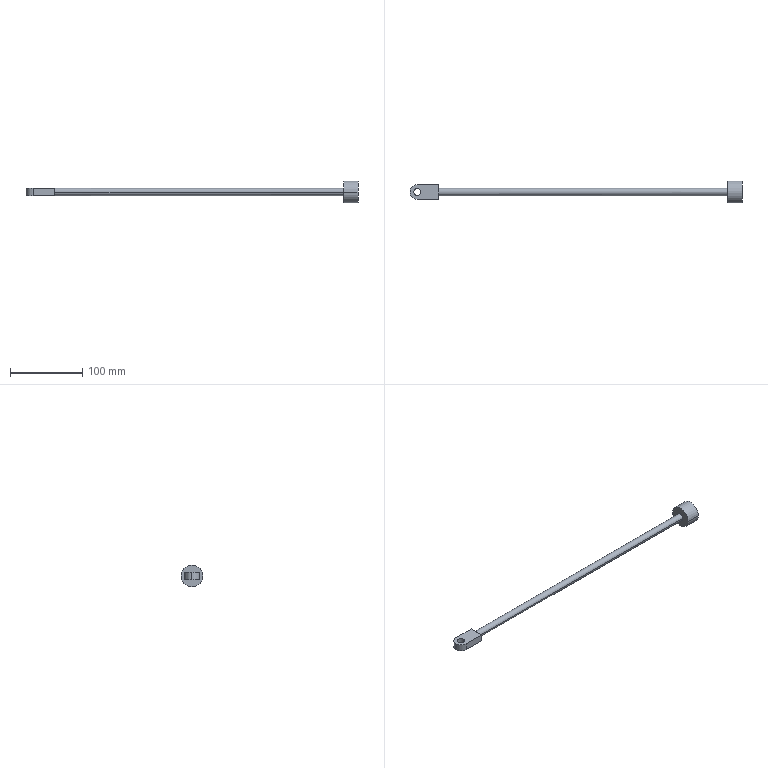Part | SolidWorks | features Extrusion 1, Revolution 1 | 1 solid | 16 faces | box 460 x 30 x 30 mm | volume 52338 mm3 | cylinder 8 | plane 8 | commonest cylinder face diameters 10 x4 20 x2 30 x2
STEP:
#1=CARTESIAN_POINT('',(430.,15.,0.));
#2=VERTEX_POINT('',#1);
#3=CARTESIAN_POINT('',(430.,-15.,0.));
#4=VERTEX_POINT('',#3);
#5=CARTESIAN_POINT('',(430.,0.,0.));
#6=DIRECTION('',(1.,0.,0.));
#7=DIRECTION('',(0.,1.,0.));
#8=AXIS2_PLACEMENT_3D('',#5,#6,#7);
#9=CIRCLE('',#8,15.);
#10=EDGE_CURVE('',#2,#4,#9,.T.);
#11=ORIENTED_EDGE('',*,*,#10,.T.);
#12=CARTESIAN_POINT('',(450.,-15.,0.));
#13=VERTEX_POINT('',#12);
#14=CARTESIAN_POINT('',(450.,-15.,0.));
#15=DIRECTION('',(1.,0.,0.));
#16=VECTOR('',#15,1000.);
#17=LINE('',#14,#16);
#18=EDGE_CURVE('',#4,#13,#17,.T.);
#19=ORIENTED_EDGE('',*,*,#18,.T.);
#20=CARTESIAN_POINT('',(450.,15.,0.));
#21=VERTEX_POINT('',#20);
#22=CARTESIAN_POINT('',(450.,0.,0.));
#23=DIRECTION('',(1.,0.,0.));
#24=DIRECTION('',(0.,1.,0.));
#25=AXIS2_PLACEMENT_3D('',#22,#23,#24);
#26=CIRCLE('',#25,15.);
#27=EDGE_CURVE('',#21,#13,#26,.T.);
#28=ORIENTED_EDGE('',*,*,#27,.F.);
#29=CARTESIAN_POINT('',(450.,15.,0.));
#30=DIRECTION('',(1.,0.,0.));
#31=VECTOR('',#30,1000.);
#32=LINE('',#29,#31);
#33=EDGE_CURVE('',#2,#21,#32,.T.);
#34=ORIENTED_EDGE('',*,*,#33,.F.);
#35=EDGE_LOOP('',(#11,#19,#28,#34));
#36=FACE_OUTER_BOUND('',#35,.T.);
#37=CARTESIAN_POINT('',(450.,0.,0.));
#38=DIRECTION('',(1.,0.,0.));
#39=DIRECTION('',(0.,1.,0.));
#40=AXIS2_PLACEMENT_3D('',#37,#38,#39);
#41=CYLINDRICAL_SURFACE('',#40,15.);
#42=ADVANCED_FACE('',(#36),#41,.T.);
#43=CARTESIAN_POINT('',(30.,0.,5.));
#44=VERTEX_POINT('',#43);
#45=CARTESIAN_POINT('',(30.,-5.,0.));
#46=VERTEX_POINT('',#45);
#47=CARTESIAN_POINT('',(30.,0.,0.));
#48=DIRECTION('',(1.,0.,0.));
#49=DIRECTION('',(0.,1.,0.));
#50=AXIS2_PLACEMENT_3D('',#47,#48,#49);
#51=CIRCLE('',#50,5.);
#52=EDGE_CURVE('',#44,#46,#51,.T.);
#53=ORIENTED_EDGE('',*,*,#52,.T.);
#54=CARTESIAN_POINT('',(430.,-5.,0.));
#55=VERTEX_POINT('',#54);
#56=CARTESIAN_POINT('',(450.,-5.,0.));
#57=DIRECTION('',(1.,0.,0.));
#58=VECTOR('',#57,1000.);
#59=LINE('',#56,#58);
#60=EDGE_CURVE('',#46,#55,#59,.T.);
#61=ORIENTED_EDGE('',*,*,#60,.T.);
#62=CARTESIAN_POINT('',(430.,5.,0.));
#63=VERTEX_POINT('',#62);
#64=CARTESIAN_POINT('',(430.,0.,0.));
#65=DIRECTION('',(1.,0.,0.));
#66=DIRECTION('',(0.,1.,0.));
#67=AXIS2_PLACEMENT_3D('',#64,#65,#66);
#68=CIRCLE('',#67,5.);
#69=EDGE_CURVE('',#63,#55,#68,.T.);
#70=ORIENTED_EDGE('',*,*,#69,.F.);
#71=CARTESIAN_POINT('',(30.,5.,0.));
#72=VERTEX_POINT('',#71);
#73=CARTESIAN_POINT('',(450.,5.,0.));
#74=DIRECTION('',(1.,0.,0.));
#75=VECTOR('',#74,1000.);
#76=LINE('',#73,#75);
#77=EDGE_CURVE('',#72,#63,#76,.T.);
#78=ORIENTED_EDGE('',*,*,#77,.F.);
#79=CARTESIAN_POINT('',(30.,0.,0.));
#80=DIRECTION('',(1.,0.,0.));
#81=DIRECTION('',(0.,1.,0.));
#82=AXIS2_PLACEMENT_3D('',#79,#80,#81);
#83=CIRCLE('',#82,5.);
#84=EDGE_CURVE('',#72,#44,#83,.T.);
#85=ORIENTED_EDGE('',*,*,#84,.T.);
#86=EDGE_LOOP('',(#53,#61,#70,#78,#85));
#87=FACE_OUTER_BOUND('',#86,.T.);
#88=CARTESIAN_POINT('',(450.,0.,0.));
#89=DIRECTION('',(1.,0.,0.));
#90=DIRECTION('',(0.,1.,0.));
#91=AXIS2_PLACEMENT_3D('',#88,#89,#90);
#92=CYLINDRICAL_SURFACE('',#91,5.);
#93=ADVANCED_FACE('',(#87),#92,.T.);
#94=CARTESIAN_POINT('',(-5.,0.,5.));
#95=VERTEX_POINT('',#94);
#96=CARTESIAN_POINT('',(5.,0.,5.));
#97=VERTEX_POINT('',#96);
#98=CARTESIAN_POINT('',(0.,0.,5.));
#99=DIRECTION('',(0.,0.,1.));
#100=DIRECTION('',(1.,0.,0.));
#101=AXIS2_PLACEMENT_3D('',#98,#99,#100);
#102=CIRCLE('',#101,5.);
#103=EDGE_CURVE('',#95,#97,#102,.T.);
#104=ORIENTED_EDGE('',*,*,#103,.T.);
#105=CARTESIAN_POINT('',(5.,0.,-5.));
#106=VERTEX_POINT('',#105);
#107=CARTESIAN_POINT('',(5.,0.,5.));
#108=DIRECTION('',(0.,0.,-1.));
#109=VECTOR('',#108,1000.);
#110=LINE('',#107,#109);
#111=EDGE_CURVE('',#97,#106,#110,.T.);
#112=ORIENTED_EDGE('',*,*,#111,.T.);
#113=CARTESIAN_POINT('',(-5.,0.,-5.));
#114=VERTEX_POINT('',#113);
#115=CARTESIAN_POINT('',(0.,0.,-5.));
#116=DIRECTION('',(0.,0.,1.));
#117=DIRECTION('',(1.,0.,0.));
#118=AXIS2_PLACEMENT_3D('',#115,#116,#117);
#119=CIRCLE('',#118,5.);
#120=EDGE_CURVE('',#114,#106,#119,.T.);
#121=ORIENTED_EDGE('',*,*,#120,.F.);
#122=CARTESIAN_POINT('',(-5.,0.,5.));
#123=DIRECTION('',(0.,0.,-1.));
#124=VECTOR('',#123,1000.);
#125=LINE('',#122,#124);
#126=EDGE_CURVE('',#95,#114,#125,.T.);
#127=ORIENTED_EDGE('',*,*,#126,.F.);
#128=EDGE_LOOP('',(#104,#112,#121,#127));
#129=FACE_OUTER_BOUND('',#128,.T.);
#130=CARTESIAN_POINT('',(0.,0.,5.));
#131=DIRECTION('',(0.,0.,-1.));
#132=DIRECTION('',(-1.,0.,0.));
#133=AXIS2_PLACEMENT_3D('',#130,#131,#132);
#134=CYLINDRICAL_SURFACE('',#133,5.);
#135=ADVANCED_FACE('',(#129),#134,.F.);
#136=CARTESIAN_POINT('',(-10.,0.,5.));
#137=VERTEX_POINT('',#136);
#138=CARTESIAN_POINT('',(0.,-10.,5.));
#139=VERTEX_POINT('',#138);
#140=CARTESIAN_POINT('',(0.,0.,5.));
#141=DIRECTION('',(0.,0.,1.));
#142=DIRECTION('',(1.,0.,0.));
#143=AXIS2_PLACEMENT_3D('',#140,#141,#142);
#144=CIRCLE('',#143,10.);
#145=EDGE_CURVE('',#137,#139,#144,.T.);
#146=ORIENTED_EDGE('',*,*,#145,.F.);
#147=CARTESIAN_POINT('',(-10.,0.,-5.));
#148=VERTEX_POINT('',#147);
#149=CARTESIAN_POINT('',(-10.,0.,5.));
#150=DIRECTION('',(0.,0.,-1.));
#151=VECTOR('',#150,1000.);
#152=LINE('',#149,#151);
#153=EDGE_CURVE('',#137,#148,#152,.T.);
#154=ORIENTED_EDGE('',*,*,#153,.T.);
#155=CARTESIAN_POINT('',(0.,-10.,-5.));
#156=VERTEX_POINT('',#155);
#157=CARTESIAN_POINT('',(0.,0.,-5.));
#158=DIRECTION('',(0.,0.,1.));
#159=DIRECTION('',(1.,0.,0.));
#160=AXIS2_PLACEMENT_3D('',#157,#158,#159);
#161=CIRCLE('',#160,10.);
#162=EDGE_CURVE('',#148,#156,#161,.T.);
#163=ORIENTED_EDGE('',*,*,#162,.T.);
#164=CARTESIAN_POINT('',(0.,-10.,5.));
#165=DIRECTION('',(0.,0.,-1.));
#166=VECTOR('',#165,1000.);
#167=LINE('',#164,#166);
#168=EDGE_CURVE('',#139,#156,#167,.T.);
#169=ORIENTED_EDGE('',*,*,#168,.F.);
#170=EDGE_LOOP('',(#146,#154,#163,#169));
#171=FACE_OUTER_BOUND('',#170,.T.);
#172=CARTESIAN_POINT('',(0.,0.,5.));
#173=DIRECTION('',(0.,0.,-1.));
#174=DIRECTION('',(-1.,0.,0.));
#175=AXIS2_PLACEMENT_3D('',#172,#173,#174);
#176=CYLINDRICAL_SURFACE('',#175,10.);
#177=ADVANCED_FACE('',(#171),#176,.T.);
#178=ORIENTED_EDGE('',*,*,#52,.F.);
#179=CARTESIAN_POINT('',(30.,-10.,5.));
#180=VERTEX_POINT('',#179);
#181=CARTESIAN_POINT('',(30.,10.,5.));
#182=DIRECTION('',(0.,1.,0.));
#183=VECTOR('',#182,1000.);
#184=LINE('',#181,#183);
#185=EDGE_CURVE('',#180,#44,#184,.T.);
#186=ORIENTED_EDGE('',*,*,#185,.F.);
#187=CARTESIAN_POINT('',(30.,-10.,-5.));
#188=VERTEX_POINT('',#187);
#189=CARTESIAN_POINT('',(30.,-10.,5.));
#190=DIRECTION('',(0.,0.,-1.));
#191=VECTOR('',#190,1000.);
#192=LINE('',#189,#191);
#193=EDGE_CURVE('',#180,#188,#192,.T.);
#194=ORIENTED_EDGE('',*,*,#193,.T.);
#195=CARTESIAN_POINT('',(30.,0.,-5.));
#196=VERTEX_POINT('',#195);
#197=CARTESIAN_POINT('',(30.,10.,-5.));
#198=DIRECTION('',(0.,1.,0.));
#199=VECTOR('',#198,1000.);
#200=LINE('',#197,#199);
#201=EDGE_CURVE('',#188,#196,#200,.T.);
#202=ORIENTED_EDGE('',*,*,#201,.T.);
#203=CARTESIAN_POINT('',(30.,0.,0.));
#204=DIRECTION('',(1.,0.,0.));
#205=DIRECTION('',(0.,1.,0.));
#206=AXIS2_PLACEMENT_3D('',#203,#204,#205);
#207=CIRCLE('',#206,5.);
#208=EDGE_CURVE('',#46,#196,#207,.T.);
#209=ORIENTED_EDGE('',*,*,#208,.F.);
#210=EDGE_LOOP('',(#178,#186,#194,#202,#209));
#211=FACE_OUTER_BOUND('',#210,.T.);
#212=CARTESIAN_POINT('',(30.,10.,5.));
#213=DIRECTION('',(-1.,0.,0.));
#214=DIRECTION('',(0.,0.,1.));
#215=AXIS2_PLACEMENT_3D('',#212,#213,#214);
#216=PLANE('',#215);
#217=ADVANCED_FACE('',(#211),#216,.F.);
#218=CARTESIAN_POINT('',(30.,0.,0.));
#219=DIRECTION('',(1.,0.,0.));
#220=DIRECTION('',(0.,1.,0.));
#221=AXIS2_PLACEMENT_3D('',#218,#219,#220);
#222=CIRCLE('',#221,5.);
#223=EDGE_CURVE('',#196,#72,#222,.T.);
#224=ORIENTED_EDGE('',*,*,#223,.F.);
#225=CARTESIAN_POINT('',(30.,10.,-5.));
#226=VERTEX_POINT('',#225);
#227=CARTESIAN_POINT('',(30.,10.,-5.));
#228=DIRECTION('',(0.,1.,0.));
#229=VECTOR('',#228,1000.);
#230=LINE('',#227,#229);
#231=EDGE_CURVE('',#196,#226,#230,.T.);
#232=ORIENTED_EDGE('',*,*,#231,.T.);
#233=CARTESIAN_POINT('',(30.,10.,5.));
#234=VERTEX_POINT('',#233);
#235=CARTESIAN_POINT('',(30.,10.,5.));
#236=DIRECTION('',(0.,0.,-1.));
#237=VECTOR('',#236,1000.);
#238=LINE('',#235,#237);
#239=EDGE_CURVE('',#234,#226,#238,.T.);
#240=ORIENTED_EDGE('',*,*,#239,.F.);
#241=CARTESIAN_POINT('',(30.,10.,5.));
#242=DIRECTION('',(0.,1.,0.));
#243=VECTOR('',#242,1000.);
#244=LINE('',#241,#243);
#245=EDGE_CURVE('',#44,#234,#244,.T.);
#246=ORIENTED_EDGE('',*,*,#245,.F.);
#247=ORIENTED_EDGE('',*,*,#84,.F.);
#248=EDGE_LOOP('',(#224,#232,#240,#246,#247));
#249=FACE_OUTER_BOUND('',#248,.T.);
#250=CARTESIAN_POINT('',(30.,10.,5.));
#251=DIRECTION('',(-1.,0.,0.));
#252=DIRECTION('',(0.,0.,1.));
#253=AXIS2_PLACEMENT_3D('',#250,#251,#252);
#254=PLANE('',#253);
#255=ADVANCED_FACE('',(#249),#254,.F.);
#256=CARTESIAN_POINT('',(0.,10.,5.));
#257=VERTEX_POINT('',#256);
#258=CARTESIAN_POINT('',(0.,0.,5.));
#259=DIRECTION('',(0.,0.,1.));
#260=DIRECTION('',(1.,0.,0.));
#261=AXIS2_PLACEMENT_3D('',#258,#259,#260);
#262=CIRCLE('',#261,10.);
#263=EDGE_CURVE('',#257,#137,#262,.T.);
#264=ORIENTED_EDGE('',*,*,#263,.T.);
#265=ORIENTED_EDGE('',*,*,#145,.T.);
#266=CARTESIAN_POINT('',(30.,-10.,5.));
#267=DIRECTION('',(1.,0.,0.));
#268=VECTOR('',#267,1000.);
#269=LINE('',#266,#268);
#270=EDGE_CURVE('',#139,#180,#269,.T.);
#271=ORIENTED_EDGE('',*,*,#270,.T.);
#272=ORIENTED_EDGE('',*,*,#185,.T.);
#273=ORIENTED_EDGE('',*,*,#245,.T.);
#274=CARTESIAN_POINT('',(0.,10.,5.));
#275=DIRECTION('',(-1.,0.,0.));
#276=VECTOR('',#275,1000.);
#277=LINE('',#274,#276);
#278=EDGE_CURVE('',#234,#257,#277,.T.);
#279=ORIENTED_EDGE('',*,*,#278,.T.);
#280=EDGE_LOOP('',(#264,#265,#271,#272,#273,#279));
#281=FACE_OUTER_BOUND('',#280,.T.);
#282=ORIENTED_EDGE('',*,*,#103,.F.);
#283=CARTESIAN_POINT('',(0.,0.,5.));
#284=DIRECTION('',(0.,0.,1.));
#285=DIRECTION('',(1.,0.,0.));
#286=AXIS2_PLACEMENT_3D('',#283,#284,#285);
#287=CIRCLE('',#286,5.);
#288=EDGE_CURVE('',#97,#95,#287,.T.);
#289=ORIENTED_EDGE('',*,*,#288,.F.);
#290=EDGE_LOOP('',(#282,#289));
#291=FACE_BOUND('',#290,.T.);
#292=CARTESIAN_POINT('',(0.,0.,5.));
#293=DIRECTION('',(0.,0.,1.));
#294=DIRECTION('',(1.,0.,0.));
#295=AXIS2_PLACEMENT_3D('',#292,#293,#294);
#296=PLANE('',#295);
#297=ADVANCED_FACE('',(#281,#291),#296,.T.);
#298=CARTESIAN_POINT('',(0.,10.,-5.));
#299=VERTEX_POINT('',#298);
#300=CARTESIAN_POINT('',(0.,0.,-5.));
#301=DIRECTION('',(0.,0.,1.));
#302=DIRECTION('',(1.,0.,0.));
#303=AXIS2_PLACEMENT_3D('',#300,#301,#302);
#304=CIRCLE('',#303,10.);
#305=EDGE_CURVE('',#299,#148,#304,.T.);
#306=ORIENTED_EDGE('',*,*,#305,.F.);
#307=CARTESIAN_POINT('',(0.,10.,-5.));
#308=DIRECTION('',(-1.,0.,0.));
#309=VECTOR('',#308,1000.);
#310=LINE('',#307,#309);
#311=EDGE_CURVE('',#226,#299,#310,.T.);
#312=ORIENTED_EDGE('',*,*,#311,.F.);
#313=ORIENTED_EDGE('',*,*,#231,.F.);
#314=ORIENTED_EDGE('',*,*,#201,.F.);
#315=CARTESIAN_POINT('',(30.,-10.,-5.));
#316=DIRECTION('',(1.,0.,0.));
#317=VECTOR('',#316,1000.);
#318=LINE('',#315,#317);
#319=EDGE_CURVE('',#156,#188,#318,.T.);
#320=ORIENTED_EDGE('',*,*,#319,.F.);
#321=ORIENTED_EDGE('',*,*,#162,.F.);
#322=EDGE_LOOP('',(#306,#312,#313,#314,#320,#321));
#323=FACE_OUTER_BOUND('',#322,.T.);
#324=ORIENTED_EDGE('',*,*,#120,.T.);
#325=CARTESIAN_POINT('',(0.,0.,-5.));
#326=DIRECTION('',(0.,0.,1.));
#327=DIRECTION('',(1.,0.,0.));
#328=AXIS2_PLACEMENT_3D('',#325,#326,#327);
#329=CIRCLE('',#328,5.);
#330=EDGE_CURVE('',#106,#114,#329,.T.);
#331=ORIENTED_EDGE('',*,*,#330,.T.);
#332=EDGE_LOOP('',(#324,#331));
#333=FACE_BOUND('',#332,.T.);
#334=CARTESIAN_POINT('',(0.,0.,-5.));
#335=DIRECTION('',(0.,0.,1.));
#336=DIRECTION('',(1.,0.,0.));
#337=AXIS2_PLACEMENT_3D('',#334,#335,#336);
#338=PLANE('',#337);
#339=ADVANCED_FACE('',(#323,#333),#338,.F.);
#340=ORIENTED_EDGE('',*,*,#153,.F.);
#341=ORIENTED_EDGE('',*,*,#263,.F.);
#342=CARTESIAN_POINT('',(0.,10.,5.));
#343=DIRECTION('',(0.,0.,-1.));
#344=VECTOR('',#343,1000.);
#345=LINE('',#342,#344);
#346=EDGE_CURVE('',#257,#299,#345,.T.);
#347=ORIENTED_EDGE('',*,*,#346,.T.);
#348=ORIENTED_EDGE('',*,*,#305,.T.);
#349=EDGE_LOOP('',(#340,#341,#347,#348));
#350=FACE_OUTER_BOUND('',#349,.T.);
#351=CARTESIAN_POINT('',(0.,0.,5.));
#352=DIRECTION('',(0.,0.,-1.));
#353=DIRECTION('',(-1.,0.,0.));
#354=AXIS2_PLACEMENT_3D('',#351,#352,#353);
#355=CYLINDRICAL_SURFACE('',#354,10.);
#356=ADVANCED_FACE('',(#350),#355,.T.);
#357=ORIENTED_EDGE('',*,*,#319,.T.);
#358=ORIENTED_EDGE('',*,*,#193,.F.);
#359=ORIENTED_EDGE('',*,*,#270,.F.);
#360=ORIENTED_EDGE('',*,*,#168,.T.);
#361=EDGE_LOOP('',(#357,#358,#359,#360));
#362=FACE_OUTER_BOUND('',#361,.T.);
#363=CARTESIAN_POINT('',(30.,-10.,5.));
#364=DIRECTION('',(0.,1.,0.));
#365=DIRECTION('',(-1.,0.,0.));
#366=AXIS2_PLACEMENT_3D('',#363,#364,#365);
#367=PLANE('',#366);
#368=ADVANCED_FACE('',(#362),#367,.F.);
#369=ORIENTED_EDGE('',*,*,#311,.T.);
#370=ORIENTED_EDGE('',*,*,#346,.F.);
#371=ORIENTED_EDGE('',*,*,#278,.F.);
#372=ORIENTED_EDGE('',*,*,#239,.T.);
#373=EDGE_LOOP('',(#369,#370,#371,#372));
#374=FACE_OUTER_BOUND('',#373,.T.);
#375=CARTESIAN_POINT('',(0.,10.,5.));
#376=DIRECTION('',(0.,-1.,0.));
#377=DIRECTION('',(1.,0.,0.));
#378=AXIS2_PLACEMENT_3D('',#375,#376,#377);
#379=PLANE('',#378);
#380=ADVANCED_FACE('',(#374),#379,.F.);
#381=ORIENTED_EDGE('',*,*,#111,.F.);
#382=ORIENTED_EDGE('',*,*,#288,.T.);
#383=ORIENTED_EDGE('',*,*,#126,.T.);
#384=ORIENTED_EDGE('',*,*,#330,.F.);
#385=EDGE_LOOP('',(#381,#382,#383,#384));
#386=FACE_OUTER_BOUND('',#385,.T.);
#387=CARTESIAN_POINT('',(0.,0.,5.));
#388=DIRECTION('',(0.,0.,-1.));
#389=DIRECTION('',(-1.,0.,0.));
#390=AXIS2_PLACEMENT_3D('',#387,#388,#389);
#391=CYLINDRICAL_SURFACE('',#390,5.);
#392=ADVANCED_FACE('',(#386),#391,.F.);
#393=ORIENTED_EDGE('',*,*,#60,.F.);
#394=ORIENTED_EDGE('',*,*,#208,.T.);
#395=ORIENTED_EDGE('',*,*,#223,.T.);
#396=ORIENTED_EDGE('',*,*,#77,.T.);
#397=CARTESIAN_POINT('',(430.,0.,0.));
#398=DIRECTION('',(1.,0.,0.));
#399=DIRECTION('',(0.,1.,0.));
#400=AXIS2_PLACEMENT_3D('',#397,#398,#399);
#401=CIRCLE('',#400,5.);
#402=EDGE_CURVE('',#55,#63,#401,.T.);
#403=ORIENTED_EDGE('',*,*,#402,.F.);
#404=EDGE_LOOP('',(#393,#394,#395,#396,#403));
#405=FACE_OUTER_BOUND('',#404,.T.);
#406=CARTESIAN_POINT('',(450.,0.,0.));
#407=DIRECTION('',(1.,0.,0.));
#408=DIRECTION('',(0.,1.,0.));
#409=AXIS2_PLACEMENT_3D('',#406,#407,#408);
#410=CYLINDRICAL_SURFACE('',#409,5.);
#411=ADVANCED_FACE('',(#405),#410,.T.);
#412=ORIENTED_EDGE('',*,*,#10,.F.);
#413=CARTESIAN_POINT('',(430.,0.,0.));
#414=DIRECTION('',(1.,0.,0.));
#415=DIRECTION('',(0.,1.,0.));
#416=AXIS2_PLACEMENT_3D('',#413,#414,#415);
#417=CIRCLE('',#416,15.);
#418=EDGE_CURVE('',#4,#2,#417,.T.);
#419=ORIENTED_EDGE('',*,*,#418,.F.);
#420=EDGE_LOOP('',(#412,#419));
#421=FACE_OUTER_BOUND('',#420,.T.);
#422=ORIENTED_EDGE('',*,*,#69,.T.);
#423=ORIENTED_EDGE('',*,*,#402,.T.);
#424=EDGE_LOOP('',(#422,#423));
#425=FACE_BOUND('',#424,.T.);
#426=CARTESIAN_POINT('',(430.,-5.,0.));
#427=DIRECTION('',(1.,0.,0.));
#428=DIRECTION('',(0.,1.,0.));
#429=AXIS2_PLACEMENT_3D('',#426,#427,#428);
#430=PLANE('',#429);
#431=ADVANCED_FACE('',(#421,#425),#430,.F.);
#432=ORIENTED_EDGE('',*,*,#18,.F.);
#433=ORIENTED_EDGE('',*,*,#418,.T.);
#434=ORIENTED_EDGE('',*,*,#33,.T.);
#435=CARTESIAN_POINT('',(450.,0.,0.));
#436=DIRECTION('',(1.,0.,0.));
#437=DIRECTION('',(0.,1.,0.));
#438=AXIS2_PLACEMENT_3D('',#435,#436,#437);
#439=CIRCLE('',#438,15.);
#440=EDGE_CURVE('',#13,#21,#439,.T.);
#441=ORIENTED_EDGE('',*,*,#440,.F.);
#442=EDGE_LOOP('',(#432,#433,#434,#441));
#443=FACE_OUTER_BOUND('',#442,.T.);
#444=CARTESIAN_POINT('',(450.,0.,0.));
#445=DIRECTION('',(1.,0.,0.));
#446=DIRECTION('',(0.,1.,0.));
#447=AXIS2_PLACEMENT_3D('',#444,#445,#446);
#448=CYLINDRICAL_SURFACE('',#447,15.);
#449=ADVANCED_FACE('',(#443),#448,.T.);
#450=ORIENTED_EDGE('',*,*,#27,.T.);
#451=ORIENTED_EDGE('',*,*,#440,.T.);
#452=EDGE_LOOP('',(#450,#451));
#453=FACE_OUTER_BOUND('',#452,.T.);
#454=CARTESIAN_POINT('',(450.,-15.,0.));
#455=DIRECTION('',(-1.,0.,0.));
#456=DIRECTION('',(0.,-1.,0.));
#457=AXIS2_PLACEMENT_3D('',#454,#455,#456);
#458=PLANE('',#457);
#459=ADVANCED_FACE('',(#453),#458,.F.);
#460=CLOSED_SHELL('',(#42,#93,#135,#177,#217,#255,#297,#339,#356,#368,#380,#392,#411,#431,#449,#459));
#461=MANIFOLD_SOLID_BREP('',#460);
#462=CARTESIAN_POINT('',(0.,0.,0.));
#463=DIRECTION('',(0.,0.,1.));
#464=DIRECTION('',(1.,0.,0.));
#465=AXIS2_PLACEMENT_3D('',#462,#463,#464);
#466=(LENGTH_UNIT()NAMED_UNIT(*)SI_UNIT(.MILLI.,.METRE.));
#467=UNCERTAINTY_MEASURE_WITH_UNIT(LENGTH_MEASURE(0.00001),#466,'','');
#468=(NAMED_UNIT(*)PLANE_ANGLE_UNIT()SI_UNIT($,.RADIAN.));
#469=(NAMED_UNIT(*)SI_UNIT($,.STERADIAN.)SOLID_ANGLE_UNIT());
#470=(GEOMETRIC_REPRESENTATION_CONTEXT(3)GLOBAL_UNCERTAINTY_ASSIGNED_CONTEXT((#467))GLOBAL_UNIT_ASSIGNED_CONTEXT((#466,#468,#469))REPRESENTATION_CONTEXT('',''));
#471=ADVANCED_BREP_SHAPE_REPRESENTATION('',(#461,#465),#470);